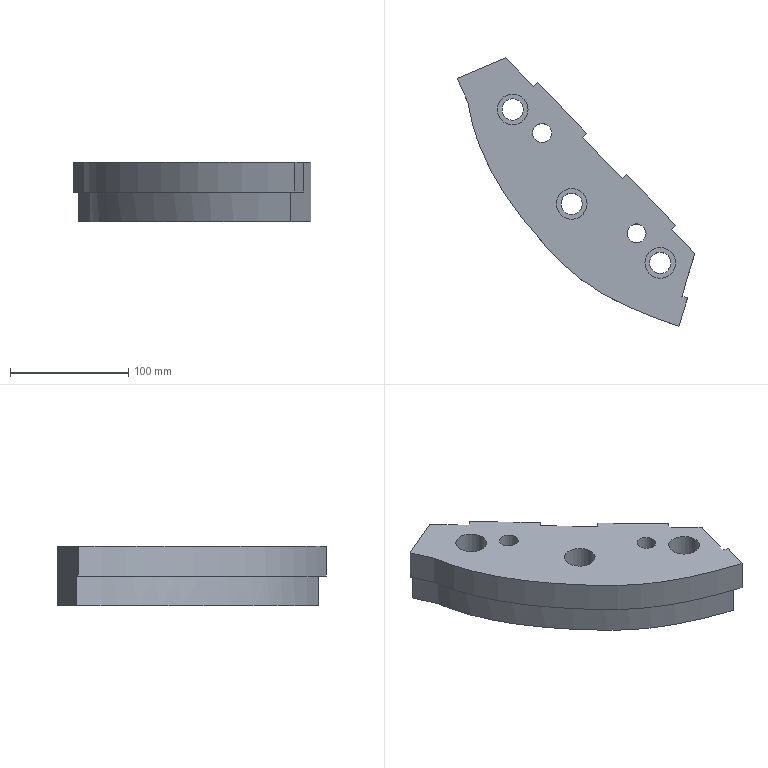Part | NX | features solid 2 | 1 solid | 29 faces | box 201.367 x 227.4 x 50 mm | volume 876647 mm3 | plane 18 | cylinder 8 | spline 3 | commonest cylinder face diameters 18 x3 26 x3 16 x2
STEP:
#1=CARTESIAN_POINT('',(-598.221,-127.253,-50.));
#2=VERTEX_POINT('',#1);
#3=CARTESIAN_POINT('',(-606.221,-127.253,-50.));
#4=DIRECTION('',(0.,0.,1.));
#5=DIRECTION('',(1.,0.,0.));
#6=AXIS2_PLACEMENT_3D('',#3,#4,#5);
#7=CIRCLE('',#6,8.);
#8=EDGE_CURVE('',#2,#2,#7,.F.);
#9=ORIENTED_EDGE('',*,*,#8,.F.);
#10=EDGE_LOOP('',(#9));
#11=FACE_BOUND('',#10,.T.);
#12=CARTESIAN_POINT('',(-678.221,-42.253,-50.));
#13=VERTEX_POINT('',#12);
#14=CARTESIAN_POINT('',(-686.221,-42.253,-50.));
#15=DIRECTION('',(0.,0.,1.));
#16=DIRECTION('',(1.,0.,0.));
#17=AXIS2_PLACEMENT_3D('',#14,#15,#16);
#18=CIRCLE('',#17,8.);
#19=EDGE_CURVE('',#13,#13,#18,.F.);
#20=ORIENTED_EDGE('',*,*,#19,.F.);
#21=EDGE_LOOP('',(#20));
#22=FACE_BOUND('',#21,.T.);
#23=CARTESIAN_POINT('',(-753.635,6.009,-50.));
#24=VERTEX_POINT('',#23);
#25=CARTESIAN_POINT('',(-717.151,21.495,-50.));
#26=VERTEX_POINT('',#25);
#27=CARTESIAN_POINT('',(-1088.176,-135.995,-50.));
#28=DIRECTION('',(0.9205,0.3907,0.));
#29=VECTOR('',#28,1000.);
#30=LINE('',#27,#29);
#31=EDGE_CURVE('',#24,#26,#30,.T.);
#32=ORIENTED_EDGE('',*,*,#31,.T.);
#33=CARTESIAN_POINT('',(-693.858,-2.626,-50.));
#34=VERTEX_POINT('',#33);
#35=CARTESIAN_POINT('',(-475.644,-228.593,-50.));
#36=DIRECTION('',(0.6947,-0.7193,0.));
#37=VECTOR('',#36,1000.);
#38=LINE('',#35,#37);
#39=EDGE_CURVE('',#26,#34,#38,.T.);
#40=ORIENTED_EDGE('',*,*,#39,.T.);
#41=CARTESIAN_POINT('',(-690.261,0.8474,-50.));
#42=VERTEX_POINT('',#41);
#43=CARTESIAN_POINT('',(-683.068,7.794,-50.));
#44=DIRECTION('',(0.7193,0.6947,0.));
#45=VECTOR('',#44,1000.);
#46=LINE('',#43,#45);
#47=EDGE_CURVE('',#34,#42,#46,.T.);
#48=ORIENTED_EDGE('',*,*,#47,.T.);
#49=CARTESIAN_POINT('',(-648.581,-42.313,-50.));
#50=VERTEX_POINT('',#49);
#51=CARTESIAN_POINT('',(-472.047,-225.12,-50.));
#52=DIRECTION('',(0.6947,-0.7193,0.));
#53=VECTOR('',#52,1000.);
#54=LINE('',#51,#53);
#55=EDGE_CURVE('',#42,#50,#54,.T.);
#56=ORIENTED_EDGE('',*,*,#55,.T.);
#57=CARTESIAN_POINT('',(-652.178,-45.786,-50.));
#58=VERTEX_POINT('',#57);
#59=CARTESIAN_POINT('',(-641.388,-35.366,-50.));
#60=DIRECTION('',(0.7193,0.6947,0.));
#61=VECTOR('',#60,1000.);
#62=LINE('',#59,#61);
#63=EDGE_CURVE('',#58,#50,#62,.T.);
#64=ORIENTED_EDGE('',*,*,#63,.F.);
#65=CARTESIAN_POINT('',(-618.219,-80.952,-50.));
#66=VERTEX_POINT('',#65);
#67=CARTESIAN_POINT('',(-475.644,-228.593,-50.));
#68=DIRECTION('',(0.6947,-0.7193,0.));
#69=VECTOR('',#68,1000.);
#70=LINE('',#67,#69);
#71=EDGE_CURVE('',#58,#66,#70,.T.);
#72=ORIENTED_EDGE('',*,*,#71,.T.);
#73=CARTESIAN_POINT('',(-614.622,-77.479,-50.));
#74=VERTEX_POINT('',#73);
#75=CARTESIAN_POINT('',(-607.429,-70.532,-50.));
#76=DIRECTION('',(0.7193,0.6947,0.));
#77=VECTOR('',#76,1000.);
#78=LINE('',#75,#77);
#79=EDGE_CURVE('',#66,#74,#78,.T.);
#80=ORIENTED_EDGE('',*,*,#79,.T.);
#81=CARTESIAN_POINT('',(-572.943,-120.639,-50.));
#82=VERTEX_POINT('',#81);
#83=CARTESIAN_POINT('',(-472.047,-225.12,-50.));
#84=DIRECTION('',(0.6947,-0.7193,0.));
#85=VECTOR('',#84,1000.);
#86=LINE('',#83,#85);
#87=EDGE_CURVE('',#74,#82,#86,.T.);
#88=ORIENTED_EDGE('',*,*,#87,.T.);
#89=CARTESIAN_POINT('',(-576.539,-124.112,-50.));
#90=VERTEX_POINT('',#89);
#91=CARTESIAN_POINT('',(-565.749,-113.693,-50.));
#92=DIRECTION('',(0.7193,0.6947,0.));
#93=VECTOR('',#92,1000.);
#94=LINE('',#91,#93);
#95=EDGE_CURVE('',#90,#82,#94,.T.);
#96=ORIENTED_EDGE('',*,*,#95,.F.);
#97=CARTESIAN_POINT('',(-556.873,-144.478,-50.));
#98=VERTEX_POINT('',#97);
#99=CARTESIAN_POINT('',(-475.644,-228.593,-50.));
#100=DIRECTION('',(0.6947,-0.7193,0.));
#101=VECTOR('',#100,1000.);
#102=LINE('',#99,#101);
#103=EDGE_CURVE('',#90,#98,#102,.T.);
#104=ORIENTED_EDGE('',*,*,#103,.T.);
#105=CARTESIAN_POINT('',(-573.715,-199.565,-50.));
#106=VERTEX_POINT('',#105);
#107=CARTESIAN_POINT('',(-717.976,-671.424,-50.));
#108=DIRECTION('',(0.2924,0.9563,0.));
#109=VECTOR('',#108,1000.);
#110=LINE('',#107,#109);
#111=EDGE_CURVE('',#106,#98,#110,.T.);
#112=ORIENTED_EDGE('',*,*,#111,.F.);
#113=CARTESIAN_POINT('',(-573.715,-199.565,-50.));
#114=CARTESIAN_POINT('',(-576.788,-198.542,-50.));
#115=CARTESIAN_POINT('',(-582.785,-196.48,-50.));
#116=CARTESIAN_POINT('',(-589.908,-193.86,-50.));
#117=CARTESIAN_POINT('',(-595.383,-191.738,-50.));
#118=CARTESIAN_POINT('',(-599.375,-190.136,-50.));
#119=CARTESIAN_POINT('',(-602.617,-188.786,-50.));
#120=CARTESIAN_POINT('',(-604.821,-187.843,-50.));
#121=CARTESIAN_POINT('',(-606.091,-187.292,-50.));
#122=CARTESIAN_POINT('',(-606.968,-186.908,-50.));
#123=CARTESIAN_POINT('',(-608.1,-186.407,-50.));
#124=CARTESIAN_POINT('',(-609.511,-185.776,-50.));
#125=CARTESIAN_POINT('',(-611.998,-184.645,-50.));
#126=CARTESIAN_POINT('',(-615.464,-183.016,-50.));
#127=CARTESIAN_POINT('',(-619.529,-181.019,-50.));
#128=CARTESIAN_POINT('',(-624.805,-178.311,-50.));
#129=CARTESIAN_POINT('',(-629.881,-175.522,-50.));
#130=CARTESIAN_POINT('',(-634.12,-173.031,-50.));
#131=CARTESIAN_POINT('',(-636.521,-171.569,-50.));
#132=CARTESIAN_POINT('',(-638.21,-170.518,-50.));
#133=CARTESIAN_POINT('',(-640.201,-169.248,-50.));
#134=CARTESIAN_POINT('',(-642.698,-167.61,-50.));
#135=CARTESIAN_POINT('',(-645.779,-165.508,-50.));
#136=CARTESIAN_POINT('',(-649.35,-162.935,-50.));
#137=CARTESIAN_POINT('',(-652.753,-160.349,-50.));
#138=CARTESIAN_POINT('',(-656.212,-157.564,-50.));
#139=CARTESIAN_POINT('',(-659.605,-154.671,-50.));
#140=CARTESIAN_POINT('',(-662.395,-152.157,-50.));
#141=CARTESIAN_POINT('',(-664.343,-150.328,-50.));
#142=CARTESIAN_POINT('',(-665.429,-149.289,-50.));
#143=CARTESIAN_POINT('',(-666.302,-148.442,-50.));
#144=CARTESIAN_POINT('',(-666.938,-147.817,-50.));
#145=CARTESIAN_POINT('',(-667.89,-146.875,-50.));
#146=CARTESIAN_POINT('',(-669.556,-145.204,-50.));
#147=CARTESIAN_POINT('',(-672.079,-142.613,-50.));
#148=CARTESIAN_POINT('',(-674.748,-139.795,-50.));
#149=CARTESIAN_POINT('',(-676.713,-137.682,-50.));
#150=CARTESIAN_POINT('',(-677.842,-136.458,-50.));
#151=CARTESIAN_POINT('',(-678.75,-135.468,-50.));
#152=CARTESIAN_POINT('',(-679.481,-134.666,-50.));
#153=CARTESIAN_POINT('',(-680.512,-133.531,-50.));
#154=CARTESIAN_POINT('',(-682.275,-131.573,-50.));
#155=CARTESIAN_POINT('',(-684.778,-128.749,-50.));
#156=CARTESIAN_POINT('',(-687.216,-125.939,-50.));
#157=CARTESIAN_POINT('',(-689.168,-123.651,-50.));
#158=CARTESIAN_POINT('',(-690.541,-122.024,-50.));
#159=CARTESIAN_POINT('',(-692.193,-120.044,-50.));
#160=CARTESIAN_POINT('',(-694.26,-117.531,-50.));
#161=CARTESIAN_POINT('',(-697.843,-113.087,-50.));
#162=CARTESIAN_POINT('',(-702.701,-106.8,-50.));
#163=CARTESIAN_POINT('',(-708.165,-99.29,-50.));
#164=CARTESIAN_POINT('',(-713.251,-91.833,-50.));
#165=CARTESIAN_POINT('',(-717.962,-84.424,-50.));
#166=CARTESIAN_POINT('',(-721.573,-78.291,-50.));
#167=CARTESIAN_POINT('',(-724.275,-73.408,-50.));
#168=CARTESIAN_POINT('',(-726.206,-69.761,-50.));
#169=CARTESIAN_POINT('',(-727.742,-66.722,-50.));
#170=CARTESIAN_POINT('',(-728.767,-64.619,-50.));
#171=CARTESIAN_POINT('',(-729.354,-63.39,-50.));
#172=CARTESIAN_POINT('',(-729.751,-62.551,-50.));
#173=CARTESIAN_POINT('',(-730.287,-61.398,-50.));
#174=CARTESIAN_POINT('',(-730.94,-59.973,-50.));
#175=CARTESIAN_POINT('',(-732.076,-57.432,-50.));
#176=CARTESIAN_POINT('',(-733.601,-53.843,-50.));
#177=CARTESIAN_POINT('',(-735.301,-49.544,-50.));
#178=CARTESIAN_POINT('',(-737.383,-43.847,-50.));
#179=CARTESIAN_POINT('',(-739.193,-38.183,-50.));
#180=CARTESIAN_POINT('',(-740.536,-33.281,-50.));
#181=CARTESIAN_POINT('',(-741.239,-30.466,-50.));
#182=CARTESIAN_POINT('',(-741.719,-28.428,-50.));
#183=CARTESIAN_POINT('',(-742.22,-26.135,-50.));
#184=CARTESIAN_POINT('',(-742.668,-23.895,-50.));
#185=CARTESIAN_POINT('',(-743.085,-21.629,-50.));
#186=CARTESIAN_POINT('',(-743.4,-19.725,-50.));
#187=CARTESIAN_POINT('',(-743.636,-18.217,-50.));
#188=CARTESIAN_POINT('',(-743.802,-17.013,-50.));
#189=CARTESIAN_POINT('',(-743.972,-16.088,-50.));
#190=CARTESIAN_POINT('',(-744.359,-14.775,-50.));
#191=CARTESIAN_POINT('',(-744.695,-13.855,-50.));
#192=CARTESIAN_POINT('',(-745.193,-12.697,-50.));
#193=CARTESIAN_POINT('',(-745.585,-11.868,-50.));
#194=CARTESIAN_POINT('',(-745.882,-11.249,-50.));
#195=CARTESIAN_POINT('',(-746.037,-10.929,-50.));
#196=CARTESIAN_POINT('',(-746.198,-10.602,-50.));
#197=CARTESIAN_POINT('',(-746.192,-10.61,-50.));
#198=CARTESIAN_POINT('',(-746.298,-10.385,-50.));
#199=CARTESIAN_POINT('',(-746.421,-10.121,-50.));
#200=CARTESIAN_POINT('',(-746.539,-9.866,-50.));
#201=CARTESIAN_POINT('',(-746.666,-9.591,-50.));
#202=CARTESIAN_POINT('',(-746.708,-9.5,-50.));
#203=CARTESIAN_POINT('',(-746.794,-9.315,-50.));
#204=CARTESIAN_POINT('',(-746.893,-9.102,-50.));
#205=CARTESIAN_POINT('',(-747.01,-8.851,-50.));
#206=CARTESIAN_POINT('',(-747.146,-8.557,-50.));
#207=CARTESIAN_POINT('',(-747.205,-8.431,-50.));
#208=CARTESIAN_POINT('',(-747.331,-8.16,-50.));
#209=CARTESIAN_POINT('',(-747.51,-7.777,-50.));
#210=CARTESIAN_POINT('',(-747.773,-7.213,-50.));
#211=CARTESIAN_POINT('',(-748.214,-6.269,-50.));
#212=CARTESIAN_POINT('',(-748.706,-5.215,-50.));
#213=CARTESIAN_POINT('',(-749.228,-4.092,-50.));
#214=CARTESIAN_POINT('',(-749.59,-3.309,-50.));
#215=CARTESIAN_POINT('',(-749.861,-2.721,-50.));
#216=CARTESIAN_POINT('',(-749.995,-2.431,-50.));
#217=CARTESIAN_POINT('',(-750.304,-1.756,-50.));
#218=CARTESIAN_POINT('',(-750.644,-1.005,-50.));
#219=CARTESIAN_POINT('',(-751.249,0.341,-50.));
#220=CARTESIAN_POINT('',(-752.352,2.858,-50.));
#221=CARTESIAN_POINT('',(-753.162,4.809,-50.));
#222=CARTESIAN_POINT('',(-753.635,6.009,-50.));
#223=B_SPLINE_CURVE_WITH_KNOTS('',3,(#113,#114,#115,#116,#117,#118,#119,#120,#121,#122,#123,#124,#125,#126,#127,#128,#129,#130,#131,#132,#133,#134,#135,#136,#137,#138,#139,#140,#141,#142,#143,#144,#145,#146,#147,#148,#149,#150,#151,#152,#153,#154,#155,#156,#157,#158,#159,#160,#161,#162,#163,#164,#165,#166,#167,#168,#169,#170,#171,#172,#173,#174,#175,#176,#177,#178,#179,#180,#181,#182,#183,#184,#185,#186,#187,#188,#189,#190,#191,#192,#193,#194,#195,#196,#197,#198,#199,#200,#201,#202,#203,#204,#205,#206,#207,#208,#209,#210,#211,#212,#213,#214,#215,#216,#217,#218,#219,#220,#221,#222),.UNSPECIFIED.,.F.,.F.,(4,1,1,1,1,1,1,1,1,1,1,1,1,1,1,1,1,1,1,1,1,1,1,1,1,1,1,1,1,1,1,1,1,1,1,1,1,1,1,1,1,1,1,1,1,1,1,1,1,1,1,1,1,1,1,1,1,1,1,1,1,1,1,1,1,1,1,1,1,1,1,1,1,1,1,1,1,1,1,1,1,1,1,1,1,1,1,1,1,1,1,1,1,1,1,1,1,1,1,1,1,1,1,1,1,1,1,4),(0.,0.03125,0.0625,0.07812,0.09375,0.1094,0.1172,0.1211,0.125,0.1289,0.1328,0.1406,0.1562,0.1719,0.1875,0.2188,0.2344,0.2422,0.25,0.2578,0.2656,0.2812,0.2969,0.3125,0.3281,0.3438,0.3594,0.3672,0.3711,0.375,0.3789,0.3828,0.3906,0.4062,0.4219,0.4297,0.4336,0.4375,0.4414,0.4453,0.4531,0.4688,0.4844,0.4922,0.5,0.5078,0.5156,0.5312,0.5625,0.5938,0.625,0.6562,0.6875,0.7031,0.7188,0.7344,0.7422,0.7461,0.75,0.7539,0.7578,0.7656,0.7812,0.7969,0.8125,0.8438,0.8594,0.8672,0.875,0.8828,0.8906,0.8984,0.9062,0.9102,0.9141,0.918,0.9219,0.9258,0.9297,0.9336,0.9355,0.9365,0.9375,0.9385,0.9395,0.9404,0.9409,0.9414,0.9419,0.9424,0.9434,0.9443,0.9453,0.9463,0.9473,0.9492,0.9512,0.9531,0.957,0.9609,0.9648,0.9668,0.9688,0.9707,0.9727,0.9766,0.9844,1.),.UNSPECIFIED.);
#224=EDGE_CURVE('',#106,#24,#223,.T.);
#225=ORIENTED_EDGE('',*,*,#224,.T.);
#226=EDGE_LOOP('',(#32,#40,#48,#56,#64,#72,#80,#88,#96,#104,#112,#225));
#227=FACE_BOUND('',#226,.T.);
#228=CARTESIAN_POINT('',(-702.221,-22.253,-50.));
#229=VERTEX_POINT('',#228);
#230=CARTESIAN_POINT('',(-711.221,-22.253,-50.));
#231=DIRECTION('',(0.,0.,1.));
#232=DIRECTION('',(1.,0.,0.));
#233=AXIS2_PLACEMENT_3D('',#230,#231,#232);
#234=CIRCLE('',#233,9.);
#235=EDGE_CURVE('',#229,#229,#234,.F.);
#236=ORIENTED_EDGE('',*,*,#235,.F.);
#237=EDGE_LOOP('',(#236));
#238=FACE_BOUND('',#237,.T.);
#239=CARTESIAN_POINT('',(-652.221,-102.253,-50.));
#240=VERTEX_POINT('',#239);
#241=CARTESIAN_POINT('',(-661.221,-102.253,-50.));
#242=DIRECTION('',(0.,0.,1.));
#243=DIRECTION('',(1.,0.,0.));
#244=AXIS2_PLACEMENT_3D('',#241,#242,#243);
#245=CIRCLE('',#244,9.);
#246=EDGE_CURVE('',#240,#240,#245,.F.);
#247=ORIENTED_EDGE('',*,*,#246,.F.);
#248=EDGE_LOOP('',(#247));
#249=FACE_BOUND('',#248,.T.);
#250=CARTESIAN_POINT('',(-577.221,-152.253,-50.));
#251=VERTEX_POINT('',#250);
#252=CARTESIAN_POINT('',(-586.221,-152.253,-50.));
#253=DIRECTION('',(0.,0.,1.));
#254=DIRECTION('',(1.,0.,0.));
#255=AXIS2_PLACEMENT_3D('',#252,#253,#254);
#256=CIRCLE('',#255,9.);
#257=EDGE_CURVE('',#251,#251,#256,.F.);
#258=ORIENTED_EDGE('',*,*,#257,.F.);
#259=EDGE_LOOP('',(#258));
#260=FACE_BOUND('',#259,.T.);
#261=CARTESIAN_POINT('',(-882.213,-621.212,-50.));
#262=DIRECTION('',(0.,0.,1.));
#263=DIRECTION('',(1.,0.,0.));
#264=AXIS2_PLACEMENT_3D('',#261,#262,#263);
#265=PLANE('',#264);
#266=ADVANCED_FACE('',(#11,#22,#227,#238,#249,#260),#265,.F.);
#267=CARTESIAN_POINT('',(-618.219,-80.952,0.));
#268=VERTEX_POINT('',#267);
#269=CARTESIAN_POINT('',(-618.219,-80.952,-25.));
#270=DIRECTION('',(0.,0.,-1.));
#271=VECTOR('',#270,1000.);
#272=LINE('',#269,#271);
#273=EDGE_CURVE('',#268,#66,#272,.T.);
#274=ORIENTED_EDGE('',*,*,#273,.T.);
#275=ORIENTED_EDGE('',*,*,#71,.F.);
#276=CARTESIAN_POINT('',(-652.178,-45.786,0.));
#277=VERTEX_POINT('',#276);
#278=CARTESIAN_POINT('',(-652.178,-45.786,-25.));
#279=DIRECTION('',(0.,0.,-1.));
#280=VECTOR('',#279,1000.);
#281=LINE('',#278,#280);
#282=EDGE_CURVE('',#277,#58,#281,.T.);
#283=ORIENTED_EDGE('',*,*,#282,.F.);
#284=CARTESIAN_POINT('',(-711.018,15.144,0.));
#285=DIRECTION('',(0.6947,-0.7193,0.));
#286=VECTOR('',#285,1000.);
#287=LINE('',#284,#286);
#288=EDGE_CURVE('',#277,#268,#287,.T.);
#289=ORIENTED_EDGE('',*,*,#288,.T.);
#290=EDGE_LOOP('',(#274,#275,#283,#289));
#291=FACE_BOUND('',#290,.T.);
#292=CARTESIAN_POINT('',(-711.018,15.144,-25.));
#293=DIRECTION('',(-0.7193,-0.6947,0.));
#294=DIRECTION('',(0.6947,-0.7193,0.));
#295=AXIS2_PLACEMENT_3D('',#292,#293,#294);
#296=PLANE('',#295);
#297=ADVANCED_FACE('',(#291),#296,.F.);
#298=CARTESIAN_POINT('',(-693.858,-2.626,0.));
#299=VERTEX_POINT('',#298);
#300=CARTESIAN_POINT('',(-693.858,-2.626,-25.));
#301=DIRECTION('',(0.,0.,-1.));
#302=VECTOR('',#301,1000.);
#303=LINE('',#300,#302);
#304=EDGE_CURVE('',#299,#34,#303,.T.);
#305=ORIENTED_EDGE('',*,*,#304,.T.);
#306=ORIENTED_EDGE('',*,*,#39,.F.);
#307=CARTESIAN_POINT('',(-717.151,21.495,0.));
#308=VERTEX_POINT('',#307);
#309=CARTESIAN_POINT('',(-717.151,21.495,-25.));
#310=DIRECTION('',(0.,0.,1.));
#311=VECTOR('',#310,1000.);
#312=LINE('',#309,#311);
#313=EDGE_CURVE('',#26,#308,#312,.T.);
#314=ORIENTED_EDGE('',*,*,#313,.T.);
#315=CARTESIAN_POINT('',(-711.018,15.144,0.));
#316=DIRECTION('',(0.6947,-0.7193,0.));
#317=VECTOR('',#316,1000.);
#318=LINE('',#315,#317);
#319=EDGE_CURVE('',#308,#299,#318,.T.);
#320=ORIENTED_EDGE('',*,*,#319,.T.);
#321=EDGE_LOOP('',(#305,#306,#314,#320));
#322=FACE_BOUND('',#321,.T.);
#323=CARTESIAN_POINT('',(-711.018,15.144,-25.));
#324=DIRECTION('',(-0.7193,-0.6947,0.));
#325=DIRECTION('',(0.6947,-0.7193,0.));
#326=AXIS2_PLACEMENT_3D('',#323,#324,#325);
#327=PLANE('',#326);
#328=ADVANCED_FACE('',(#322),#327,.F.);
#329=CARTESIAN_POINT('',(-563.114,-181.994,0.));
#330=VERTEX_POINT('',#329);
#331=CARTESIAN_POINT('',(-567.865,-180.433,0.));
#332=VERTEX_POINT('',#331);
#333=CARTESIAN_POINT('',(-563.114,-181.994,0.));
#334=CARTESIAN_POINT('',(-564.701,-181.481,0.));
#335=CARTESIAN_POINT('',(-566.285,-180.961,0.));
#336=CARTESIAN_POINT('',(-567.865,-180.433,0.));
#337=B_SPLINE_CURVE_WITH_KNOTS('',3,(#333,#334,#335,#336),.UNSPECIFIED.,.F.,.F.,(4,4),(0.,0.00497),.UNSPECIFIED.);
#338=EDGE_CURVE('',#330,#332,#337,.T.);
#339=ORIENTED_EDGE('',*,*,#338,.T.);
#340=CARTESIAN_POINT('',(-556.873,-144.478,0.));
#341=VERTEX_POINT('',#340);
#342=CARTESIAN_POINT('',(-573.744,-199.661,0.));
#343=DIRECTION('',(-0.2924,-0.9563,0.));
#344=VECTOR('',#343,1000.);
#345=LINE('',#342,#344);
#346=EDGE_CURVE('',#341,#332,#345,.T.);
#347=ORIENTED_EDGE('',*,*,#346,.F.);
#348=CARTESIAN_POINT('',(-576.539,-124.112,0.));
#349=VERTEX_POINT('',#348);
#350=CARTESIAN_POINT('',(-711.018,15.144,0.));
#351=DIRECTION('',(0.6947,-0.7193,0.));
#352=VECTOR('',#351,1000.);
#353=LINE('',#350,#352);
#354=EDGE_CURVE('',#349,#341,#353,.T.);
#355=ORIENTED_EDGE('',*,*,#354,.F.);
#356=CARTESIAN_POINT('',(-572.943,-120.639,0.));
#357=VERTEX_POINT('',#356);
#358=CARTESIAN_POINT('',(-614.246,-160.525,0.));
#359=DIRECTION('',(0.7193,0.6947,0.));
#360=VECTOR('',#359,1000.);
#361=LINE('',#358,#360);
#362=EDGE_CURVE('',#349,#357,#361,.T.);
#363=ORIENTED_EDGE('',*,*,#362,.T.);
#364=CARTESIAN_POINT('',(-614.622,-77.479,0.));
#365=VERTEX_POINT('',#364);
#366=CARTESIAN_POINT('',(-611.149,-81.075,0.));
#367=DIRECTION('',(0.6947,-0.7193,0.));
#368=VECTOR('',#367,1000.);
#369=LINE('',#366,#368);
#370=EDGE_CURVE('',#365,#357,#369,.T.);
#371=ORIENTED_EDGE('',*,*,#370,.F.);
#372=CARTESIAN_POINT('',(-655.926,-117.365,0.));
#373=DIRECTION('',(0.7193,0.6947,0.));
#374=VECTOR('',#373,1000.);
#375=LINE('',#372,#374);
#376=EDGE_CURVE('',#268,#365,#375,.T.);
#377=ORIENTED_EDGE('',*,*,#376,.F.);
#378=ORIENTED_EDGE('',*,*,#288,.F.);
#379=CARTESIAN_POINT('',(-648.581,-42.313,0.));
#380=VERTEX_POINT('',#379);
#381=CARTESIAN_POINT('',(-689.885,-82.199,0.));
#382=DIRECTION('',(0.7193,0.6947,0.));
#383=VECTOR('',#382,1000.);
#384=LINE('',#381,#383);
#385=EDGE_CURVE('',#277,#380,#384,.T.);
#386=ORIENTED_EDGE('',*,*,#385,.T.);
#387=CARTESIAN_POINT('',(-690.261,0.8474,0.));
#388=VERTEX_POINT('',#387);
#389=CARTESIAN_POINT('',(-714.574,26.024,0.));
#390=DIRECTION('',(0.6947,-0.7193,0.));
#391=VECTOR('',#390,1000.);
#392=LINE('',#389,#391);
#393=EDGE_CURVE('',#388,#380,#392,.T.);
#394=ORIENTED_EDGE('',*,*,#393,.F.);
#395=CARTESIAN_POINT('',(-731.564,-39.039,0.));
#396=DIRECTION('',(0.7193,0.6947,0.));
#397=VECTOR('',#396,1000.);
#398=LINE('',#395,#397);
#399=EDGE_CURVE('',#299,#388,#398,.T.);
#400=ORIENTED_EDGE('',*,*,#399,.F.);
#401=ORIENTED_EDGE('',*,*,#319,.F.);
#402=CARTESIAN_POINT('',(-758.239,4.055,0.));
#403=VERTEX_POINT('',#402);
#404=CARTESIAN_POINT('',(-1958.229,-505.311,0.));
#405=DIRECTION('',(0.9205,0.3907,0.));
#406=VECTOR('',#405,1000.);
#407=LINE('',#404,#406);
#408=EDGE_CURVE('',#403,#308,#407,.T.);
#409=ORIENTED_EDGE('',*,*,#408,.F.);
#410=CARTESIAN_POINT('',(-570.424,-205.904,0.));
#411=VERTEX_POINT('',#410);
#412=CARTESIAN_POINT('',(-758.239,4.055,0.));
#413=CARTESIAN_POINT('',(-757.144,1.281,0.));
#414=CARTESIAN_POINT('',(-755.343,-2.817,0.));
#415=CARTESIAN_POINT('',(-752.812,-8.229,0.));
#416=CARTESIAN_POINT('',(-751.252,-11.62,0.));
#417=CARTESIAN_POINT('',(-749.959,-14.316,0.));
#418=CARTESIAN_POINT('',(-749.016,-16.348,0.));
#419=CARTESIAN_POINT('',(-748.615,-18.594,0.));
#420=CARTESIAN_POINT('',(-748.178,-21.629,0.));
#421=CARTESIAN_POINT('',(-747.492,-25.366,0.));
#422=CARTESIAN_POINT('',(-746.238,-31.284,0.));
#423=CARTESIAN_POINT('',(-744.334,-38.548,0.));
#424=CARTESIAN_POINT('',(-740.668,-49.926,0.));
#425=CARTESIAN_POINT('',(-735.009,-63.721,0.));
#426=CARTESIAN_POINT('',(-726.757,-79.698,0.));
#427=CARTESIAN_POINT('',(-717.23,-95.169,0.));
#428=CARTESIAN_POINT('',(-706.569,-110.192,0.));
#429=CARTESIAN_POINT('',(-694.918,-124.823,0.));
#430=CARTESIAN_POINT('',(-682.359,-139.091,0.));
#431=CARTESIAN_POINT('',(-669.418,-152.804,0.));
#432=CARTESIAN_POINT('',(-655.303,-165.141,0.));
#433=CARTESIAN_POINT('',(-639.796,-175.759,0.));
#434=CARTESIAN_POINT('',(-623.086,-185.082,0.));
#435=CARTESIAN_POINT('',(-600.12,-195.69,0.));
#436=CARTESIAN_POINT('',(-582.381,-202.048,0.));
#437=CARTESIAN_POINT('',(-570.424,-205.904,0.));
#438=B_SPLINE_CURVE_WITH_KNOTS('',3,(#412,#413,#414,#415,#416,#417,#418,#419,#420,#421,#422,#423,#424,#425,#426,#427,#428,#429,#430,#431,#432,#433,#434,#435,#436,#437),.UNSPECIFIED.,.F.,.F.,(4,1,1,1,1,1,1,1,1,1,1,1,1,1,1,1,1,1,1,1,1,1,1,4),(1.545,1.554,1.558,1.563,1.565,1.567,1.57,1.572,1.576,1.581,1.59,1.599,1.617,1.635,1.652,1.67,1.688,1.706,1.724,1.742,1.76,1.778,1.796,1.832),.UNSPECIFIED.);
#439=EDGE_CURVE('',#411,#403,#438,.F.);
#440=ORIENTED_EDGE('',*,*,#439,.F.);
#441=CARTESIAN_POINT('',(-976.675,-1534.691,0.));
#442=DIRECTION('',(0.2924,0.9563,0.));
#443=VECTOR('',#442,1000.);
#444=LINE('',#441,#443);
#445=EDGE_CURVE('',#411,#330,#444,.T.);
#446=ORIENTED_EDGE('',*,*,#445,.T.);
#447=EDGE_LOOP('',(#339,#347,#355,#363,#371,#377,#378,#386,#394,#400,#401,#409,#440,#446));
#448=FACE_BOUND('',#447,.T.);
#449=CARTESIAN_POINT('',(-648.221,-102.253,0.));
#450=VERTEX_POINT('',#449);
#451=CARTESIAN_POINT('',(-661.221,-102.253,0.));
#452=DIRECTION('',(0.,0.,1.));
#453=DIRECTION('',(1.,0.,0.));
#454=AXIS2_PLACEMENT_3D('',#451,#452,#453);
#455=CIRCLE('',#454,13.);
#456=EDGE_CURVE('',#450,#450,#455,.F.);
#457=ORIENTED_EDGE('',*,*,#456,.T.);
#458=EDGE_LOOP('',(#457));
#459=FACE_BOUND('',#458,.T.);
#460=CARTESIAN_POINT('',(-678.221,-42.253,0.));
#461=VERTEX_POINT('',#460);
#462=CARTESIAN_POINT('',(-686.221,-42.253,0.));
#463=DIRECTION('',(0.,0.,1.));
#464=DIRECTION('',(1.,0.,0.));
#465=AXIS2_PLACEMENT_3D('',#462,#463,#464);
#466=CIRCLE('',#465,8.);
#467=EDGE_CURVE('',#461,#461,#466,.F.);
#468=ORIENTED_EDGE('',*,*,#467,.T.);
#469=EDGE_LOOP('',(#468));
#470=FACE_BOUND('',#469,.T.);
#471=CARTESIAN_POINT('',(-598.221,-127.253,0.));
#472=VERTEX_POINT('',#471);
#473=CARTESIAN_POINT('',(-606.221,-127.253,0.));
#474=DIRECTION('',(0.,0.,1.));
#475=DIRECTION('',(1.,0.,0.));
#476=AXIS2_PLACEMENT_3D('',#473,#474,#475);
#477=CIRCLE('',#476,8.);
#478=EDGE_CURVE('',#472,#472,#477,.F.);
#479=ORIENTED_EDGE('',*,*,#478,.T.);
#480=EDGE_LOOP('',(#479));
#481=FACE_BOUND('',#480,.T.);
#482=CARTESIAN_POINT('',(-698.221,-22.253,0.));
#483=VERTEX_POINT('',#482);
#484=CARTESIAN_POINT('',(-711.221,-22.253,0.));
#485=DIRECTION('',(0.,0.,1.));
#486=DIRECTION('',(1.,0.,0.));
#487=AXIS2_PLACEMENT_3D('',#484,#485,#486);
#488=CIRCLE('',#487,13.);
#489=EDGE_CURVE('',#483,#483,#488,.F.);
#490=ORIENTED_EDGE('',*,*,#489,.T.);
#491=EDGE_LOOP('',(#490));
#492=FACE_BOUND('',#491,.T.);
#493=CARTESIAN_POINT('',(-573.221,-152.253,0.));
#494=VERTEX_POINT('',#493);
#495=CARTESIAN_POINT('',(-586.221,-152.253,0.));
#496=DIRECTION('',(0.,0.,1.));
#497=DIRECTION('',(1.,0.,0.));
#498=AXIS2_PLACEMENT_3D('',#495,#496,#497);
#499=CIRCLE('',#498,13.);
#500=EDGE_CURVE('',#494,#494,#499,.F.);
#501=ORIENTED_EDGE('',*,*,#500,.T.);
#502=EDGE_LOOP('',(#501));
#503=FACE_BOUND('',#502,.T.);
#504=CARTESIAN_POINT('',(-688.275,33.753,0.));
#505=DIRECTION('',(0.,0.,-1.));
#506=DIRECTION('',(-1.,0.,0.));
#507=AXIS2_PLACEMENT_3D('',#504,#505,#506);
#508=PLANE('',#507);
#509=ADVANCED_FACE('',(#448,#459,#470,#481,#492,#503),#508,.F.);
#510=CARTESIAN_POINT('',(-556.873,-144.478,-70.));
#511=DIRECTION('',(0.,0.,-1.));
#512=VECTOR('',#511,1000.);
#513=LINE('',#510,#512);
#514=EDGE_CURVE('',#341,#98,#513,.T.);
#515=ORIENTED_EDGE('',*,*,#514,.F.);
#516=ORIENTED_EDGE('',*,*,#346,.T.);
#517=CARTESIAN_POINT('',(-567.865,-180.433,-25.));
#518=VERTEX_POINT('',#517);
#519=CARTESIAN_POINT('',(-567.865,-180.433,-25.));
#520=DIRECTION('',(0.,0.,-1.));
#521=VECTOR('',#520,1000.);
#522=LINE('',#519,#521);
#523=EDGE_CURVE('',#518,#332,#522,.F.);
#524=ORIENTED_EDGE('',*,*,#523,.F.);
#525=CARTESIAN_POINT('',(-573.715,-199.565,-25.));
#526=VERTEX_POINT('',#525);
#527=CARTESIAN_POINT('',(-573.744,-199.661,-25.));
#528=DIRECTION('',(0.2924,0.9563,0.));
#529=VECTOR('',#528,1000.);
#530=LINE('',#527,#529);
#531=EDGE_CURVE('',#526,#518,#530,.T.);
#532=ORIENTED_EDGE('',*,*,#531,.F.);
#533=CARTESIAN_POINT('',(-573.715,-199.565,-42.5));
#534=DIRECTION('',(0.,0.,1.));
#535=VECTOR('',#534,1000.);
#536=LINE('',#533,#535);
#537=EDGE_CURVE('',#526,#106,#536,.F.);
#538=ORIENTED_EDGE('',*,*,#537,.T.);
#539=ORIENTED_EDGE('',*,*,#111,.T.);
#540=EDGE_LOOP('',(#515,#516,#524,#532,#538,#539));
#541=FACE_BOUND('',#540,.T.);
#542=CARTESIAN_POINT('',(-573.744,-199.661,-70.));
#543=DIRECTION('',(0.9563,-0.2924,0.));
#544=DIRECTION('',(0.2924,0.9563,0.));
#545=AXIS2_PLACEMENT_3D('',#542,#543,#544);
#546=PLANE('',#545);
#547=ADVANCED_FACE('',(#541),#546,.T.);
#548=CARTESIAN_POINT('',(-563.114,-181.994,-25.));
#549=VERTEX_POINT('',#548);
#550=CARTESIAN_POINT('',(-563.114,-181.994,-25.));
#551=CARTESIAN_POINT('',(-564.705,-181.48,-25.));
#552=CARTESIAN_POINT('',(-566.288,-180.96,-25.));
#553=CARTESIAN_POINT('',(-567.865,-180.433,-25.));
#554=B_SPLINE_CURVE_WITH_KNOTS('',3,(#550,#551,#552,#553),.UNSPECIFIED.,.F.,.F.,(4,4),(0.001623,0.02295),.UNSPECIFIED.);
#555=EDGE_CURVE('',#549,#518,#554,.T.);
#556=ORIENTED_EDGE('',*,*,#555,.F.);
#557=CARTESIAN_POINT('',(-570.424,-205.904,-25.));
#558=VERTEX_POINT('',#557);
#559=CARTESIAN_POINT('',(-976.675,-1534.691,-25.));
#560=DIRECTION('',(0.2924,0.9563,0.));
#561=VECTOR('',#560,1000.);
#562=LINE('',#559,#561);
#563=EDGE_CURVE('',#558,#549,#562,.T.);
#564=ORIENTED_EDGE('',*,*,#563,.F.);
#565=CARTESIAN_POINT('',(-758.239,4.055,-25.));
#566=VERTEX_POINT('',#565);
#567=CARTESIAN_POINT('',(-758.239,4.055,-25.));
#568=CARTESIAN_POINT('',(-757.142,1.278,-25.));
#569=CARTESIAN_POINT('',(-755.34,-2.825,-25.));
#570=CARTESIAN_POINT('',(-752.804,-8.244,-25.));
#571=CARTESIAN_POINT('',(-751.243,-11.64,-25.));
#572=CARTESIAN_POINT('',(-749.947,-14.338,-25.));
#573=CARTESIAN_POINT('',(-749.007,-16.374,-25.));
#574=CARTESIAN_POINT('',(-748.612,-18.625,-25.));
#575=CARTESIAN_POINT('',(-748.172,-21.66,-25.));
#576=CARTESIAN_POINT('',(-747.485,-25.4,-25.));
#577=CARTESIAN_POINT('',(-746.229,-31.321,-25.));
#578=CARTESIAN_POINT('',(-744.322,-38.591,-25.));
#579=CARTESIAN_POINT('',(-740.648,-49.978,-25.));
#580=CARTESIAN_POINT('',(-734.978,-63.788,-25.));
#581=CARTESIAN_POINT('',(-726.709,-79.784,-25.));
#582=CARTESIAN_POINT('',(-717.158,-95.277,-25.));
#583=CARTESIAN_POINT('',(-706.476,-110.316,-25.));
#584=CARTESIAN_POINT('',(-694.776,-124.992,-25.));
#585=CARTESIAN_POINT('',(-682.253,-139.205,-25.));
#586=CARTESIAN_POINT('',(-669.354,-152.867,-25.));
#587=CARTESIAN_POINT('',(-655.25,-165.181,-25.));
#588=CARTESIAN_POINT('',(-639.704,-175.817,-25.));
#589=CARTESIAN_POINT('',(-622.973,-185.138,-25.));
#590=CARTESIAN_POINT('',(-600.103,-195.693,-25.));
#591=CARTESIAN_POINT('',(-582.374,-202.05,-25.));
#592=CARTESIAN_POINT('',(-570.424,-205.904,-25.));
#593=B_SPLINE_CURVE_WITH_KNOTS('',3,(#567,#568,#569,#570,#571,#572,#573,#574,#575,#576,#577,#578,#579,#580,#581,#582,#583,#584,#585,#586,#587,#588,#589,#590,#591,#592),.UNSPECIFIED.,.F.,.F.,(4,1,1,1,1,1,1,1,1,1,1,1,1,1,1,1,1,1,1,1,1,1,1,4),(1.469,1.478,1.483,1.487,1.49,1.492,1.494,1.496,1.501,1.505,1.514,1.523,1.541,1.559,1.577,1.595,1.613,1.631,1.649,1.667,1.685,1.703,1.721,1.756),.UNSPECIFIED.);
#594=EDGE_CURVE('',#558,#566,#593,.F.);
#595=ORIENTED_EDGE('',*,*,#594,.T.);
#596=CARTESIAN_POINT('',(-753.635,6.009,-25.));
#597=VERTEX_POINT('',#596);
#598=CARTESIAN_POINT('',(-1958.229,-505.311,-25.));
#599=DIRECTION('',(0.9205,0.3907,0.));
#600=VECTOR('',#599,1000.);
#601=LINE('',#598,#600);
#602=EDGE_CURVE('',#566,#597,#601,.T.);
#603=ORIENTED_EDGE('',*,*,#602,.T.);
#604=CARTESIAN_POINT('',(-573.715,-199.565,-25.));
#605=CARTESIAN_POINT('',(-585.053,-195.791,-25.));
#606=CARTESIAN_POINT('',(-601.795,-189.572,-25.));
#607=CARTESIAN_POINT('',(-623.22,-179.362,-25.));
#608=CARTESIAN_POINT('',(-638.713,-170.517,-25.));
#609=CARTESIAN_POINT('',(-653.546,-160.162,-25.));
#610=CARTESIAN_POINT('',(-667.029,-148.094,-25.));
#611=CARTESIAN_POINT('',(-679.251,-135.061,-25.));
#612=CARTESIAN_POINT('',(-691.016,-121.671,-25.));
#613=CARTESIAN_POINT('',(-702.118,-107.769,-25.));
#614=CARTESIAN_POINT('',(-712.47,-93.281,-25.));
#615=CARTESIAN_POINT('',(-721.91,-78.111,-25.));
#616=CARTESIAN_POINT('',(-730.292,-62.032,-25.));
#617=CARTESIAN_POINT('',(-735.995,-48.165,-25.));
#618=CARTESIAN_POINT('',(-739.655,-36.74,-25.));
#619=CARTESIAN_POINT('',(-741.539,-29.452,-25.));
#620=CARTESIAN_POINT('',(-742.753,-23.514,-25.));
#621=CARTESIAN_POINT('',(-743.43,-19.773,-25.));
#622=CARTESIAN_POINT('',(-743.809,-16.72,-25.));
#623=CARTESIAN_POINT('',(-744.591,-13.815,-25.));
#624=CARTESIAN_POINT('',(-746.303,-10.453,-25.));
#625=CARTESIAN_POINT('',(-748.166,-6.348,-25.));
#626=CARTESIAN_POINT('',(-750.725,-0.9033,-25.));
#627=CARTESIAN_POINT('',(-752.534,3.221,-25.));
#628=CARTESIAN_POINT('',(-753.635,6.009,-25.));
#629=B_SPLINE_CURVE_WITH_KNOTS('',3,(#604,#605,#606,#607,#608,#609,#610,#611,#612,#613,#614,#615,#616,#617,#618,#619,#620,#621,#622,#623,#624,#625,#626,#627,#628),.UNSPECIFIED.,.F.,.F.,(4,1,1,1,1,1,1,1,1,1,1,1,1,1,1,1,1,1,1,1,1,1,4),(0.6959,0.7318,0.7497,0.7676,0.7856,0.8035,0.8214,0.8393,0.8573,0.8752,0.8931,0.9111,0.929,0.938,0.9469,0.9514,0.9559,0.9581,0.9604,0.9649,0.9693,0.9738,0.9828),.UNSPECIFIED.);
#630=EDGE_CURVE('',#526,#597,#629,.T.);
#631=ORIENTED_EDGE('',*,*,#630,.F.);
#632=ORIENTED_EDGE('',*,*,#531,.T.);
#633=EDGE_LOOP('',(#556,#564,#595,#603,#631,#632));
#634=FACE_BOUND('',#633,.T.);
#635=CARTESIAN_POINT('',(-570.424,-205.904,-25.));
#636=DIRECTION('',(0.,0.,-1.));
#637=DIRECTION('',(-1.,0.,0.));
#638=AXIS2_PLACEMENT_3D('',#635,#636,#637);
#639=PLANE('',#638);
#640=ADVANCED_FACE('',(#634),#639,.T.);
#641=ORIENTED_EDGE('',*,*,#537,.F.);
#642=ORIENTED_EDGE('',*,*,#630,.T.);
#643=CARTESIAN_POINT('',(-753.635,6.009,-42.5));
#644=DIRECTION('',(0.,0.,1.));
#645=VECTOR('',#644,1000.);
#646=LINE('',#643,#645);
#647=EDGE_CURVE('',#597,#24,#646,.F.);
#648=ORIENTED_EDGE('',*,*,#647,.T.);
#649=ORIENTED_EDGE('',*,*,#224,.F.);
#650=EDGE_LOOP('',(#641,#642,#648,#649));
#651=FACE_BOUND('',#650,.T.);
#652=CARTESIAN_POINT('',(-573.715,-199.565,-50.));
#653=CARTESIAN_POINT('',(-573.715,-199.565,-25.));
#654=CARTESIAN_POINT('',(-585.12,-195.769,-50.));
#655=CARTESIAN_POINT('',(-585.12,-195.769,-25.));
#656=CARTESIAN_POINT('',(-601.987,-189.498,-50.));
#657=CARTESIAN_POINT('',(-601.987,-189.498,-25.));
#658=CARTESIAN_POINT('',(-623.5,-179.217,-50.));
#659=CARTESIAN_POINT('',(-623.5,-179.217,-25.));
#660=CARTESIAN_POINT('',(-638.947,-170.364,-50.));
#661=CARTESIAN_POINT('',(-638.947,-170.364,-25.));
#662=CARTESIAN_POINT('',(-653.471,-160.193,-50.));
#663=CARTESIAN_POINT('',(-653.471,-160.193,-25.));
#664=CARTESIAN_POINT('',(-666.618,-148.499,-50.));
#665=CARTESIAN_POINT('',(-666.618,-148.499,-25.));
#666=CARTESIAN_POINT('',(-678.964,-135.383,-50.));
#667=CARTESIAN_POINT('',(-678.964,-135.383,-25.));
#668=CARTESIAN_POINT('',(-690.853,-121.868,-50.));
#669=CARTESIAN_POINT('',(-690.853,-121.868,-25.));
#670=CARTESIAN_POINT('',(-702.068,-107.84,-50.));
#671=CARTESIAN_POINT('',(-702.068,-107.84,-25.));
#672=CARTESIAN_POINT('',(-712.486,-93.26,-50.));
#673=CARTESIAN_POINT('',(-712.486,-93.26,-25.));
#674=CARTESIAN_POINT('',(-721.918,-78.089,-50.));
#675=CARTESIAN_POINT('',(-721.918,-78.089,-25.));
#676=CARTESIAN_POINT('',(-728.787,-64.923,-50.));
#677=CARTESIAN_POINT('',(-728.787,-64.923,-25.));
#678=CARTESIAN_POINT('',(-733.555,-54.092,-50.));
#679=CARTESIAN_POINT('',(-733.555,-54.092,-25.));
#680=CARTESIAN_POINT('',(-736.724,-45.828,-50.));
#681=CARTESIAN_POINT('',(-736.724,-45.828,-25.));
#682=CARTESIAN_POINT('',(-738.997,-38.828,-50.));
#683=CARTESIAN_POINT('',(-738.997,-38.828,-25.));
#684=CARTESIAN_POINT('',(-740.574,-33.167,-50.));
#685=CARTESIAN_POINT('',(-740.574,-33.167,-25.));
#686=CARTESIAN_POINT('',(-741.629,-28.895,-50.));
#687=CARTESIAN_POINT('',(-741.629,-28.895,-25.));
#688=CARTESIAN_POINT('',(-742.396,-25.315,-50.));
#689=CARTESIAN_POINT('',(-742.396,-25.315,-25.));
#690=CARTESIAN_POINT('',(-742.94,-22.439,-50.));
#691=CARTESIAN_POINT('',(-742.94,-22.439,-25.));
#692=CARTESIAN_POINT('',(-743.251,-20.64,-50.));
#693=CARTESIAN_POINT('',(-743.251,-20.64,-25.));
#694=CARTESIAN_POINT('',(-743.485,-19.181,-50.));
#695=CARTESIAN_POINT('',(-743.485,-19.181,-25.));
#696=CARTESIAN_POINT('',(-743.621,-18.301,-50.));
#697=CARTESIAN_POINT('',(-743.621,-18.301,-25.));
#698=CARTESIAN_POINT('',(-743.718,-17.592,-50.));
#699=CARTESIAN_POINT('',(-743.718,-17.592,-25.));
#700=CARTESIAN_POINT('',(-743.835,-16.823,-50.));
#701=CARTESIAN_POINT('',(-743.835,-16.823,-25.));
#702=CARTESIAN_POINT('',(-744.024,-15.948,-50.));
#703=CARTESIAN_POINT('',(-744.024,-15.948,-25.));
#704=CARTESIAN_POINT('',(-744.32,-14.882,-50.));
#705=CARTESIAN_POINT('',(-744.32,-14.882,-25.));
#706=CARTESIAN_POINT('',(-744.776,-13.621,-50.));
#707=CARTESIAN_POINT('',(-744.776,-13.621,-25.));
#708=CARTESIAN_POINT('',(-745.571,-11.889,-50.));
#709=CARTESIAN_POINT('',(-745.571,-11.889,-25.));
#710=CARTESIAN_POINT('',(-746.307,-10.386,-50.));
#711=CARTESIAN_POINT('',(-746.307,-10.386,-25.));
#712=CARTESIAN_POINT('',(-747.284,-8.253,-50.));
#713=CARTESIAN_POINT('',(-747.284,-8.253,-25.));
#714=CARTESIAN_POINT('',(-748.568,-5.517,-50.));
#715=CARTESIAN_POINT('',(-748.568,-5.517,-25.));
#716=CARTESIAN_POINT('',(-750.158,-2.098,-50.));
#717=CARTESIAN_POINT('',(-750.158,-2.098,-25.));
#718=CARTESIAN_POINT('',(-751.671,1.272,-50.));
#719=CARTESIAN_POINT('',(-751.671,1.272,-25.));
#720=CARTESIAN_POINT('',(-752.825,3.99,-50.));
#721=CARTESIAN_POINT('',(-752.825,3.99,-25.));
#722=CARTESIAN_POINT('',(-753.357,5.303,-50.));
#723=CARTESIAN_POINT('',(-753.357,5.303,-25.));
#724=CARTESIAN_POINT('',(-753.635,6.009,-50.));
#725=CARTESIAN_POINT('',(-753.635,6.009,-25.));
#726=B_SPLINE_SURFACE_WITH_KNOTS('',3,1,((#652,#653),(#654,#655),(#656,#657),(#658,#659),(#660,#661),(#662,#663),(#664,#665),(#666,#667),(#668,#669),(#670,#671),(#672,#673),(#674,#675),(#676,#677),(#678,#679),(#680,#681),(#682,#683),(#684,#685),(#686,#687),(#688,#689),(#690,#691),(#692,#693),(#694,#695),(#696,#697),(#698,#699),(#700,#701),(#702,#703),(#704,#705),(#706,#707),(#708,#709),(#710,#711),(#712,#713),(#714,#715),(#716,#717),(#718,#719),(#720,#721),(#722,#723),(#724,#725)),.SURF_OF_LINEAR_EXTRUSION.,.F.,.F.,.F.,(4,1,1,1,1,1,1,1,1,1,1,1,1,1,1,1,1,1,1,1,1,1,1,1,1,1,1,1,1,1,1,1,1,1,4),(2,2),(0.01729,0.1402,0.2016,0.2631,0.3245,0.386,0.4474,0.5089,0.5703,0.6318,0.6932,0.7546,0.7854,0.8161,0.8468,0.8622,0.8775,0.8929,0.9006,0.9083,0.9121,0.9159,0.9179,0.9198,0.9217,0.9236,0.9275,0.9313,0.939,0.9467,0.9543,0.9697,0.9851,0.9927,1.),(0.,1.),.UNSPECIFIED.);
#727=ADVANCED_FACE('',(#651),#726,.F.);
#728=CARTESIAN_POINT('',(-563.114,-181.994,-12.5));
#729=DIRECTION('',(0.,0.,-1.));
#730=VECTOR('',#729,1000.);
#731=LINE('',#728,#730);
#732=EDGE_CURVE('',#330,#549,#731,.T.);
#733=ORIENTED_EDGE('',*,*,#732,.F.);
#734=ORIENTED_EDGE('',*,*,#445,.F.);
#735=CARTESIAN_POINT('',(-570.424,-205.904,-70.));
#736=DIRECTION('',(0.,0.,1.));
#737=VECTOR('',#736,1000.);
#738=LINE('',#735,#737);
#739=EDGE_CURVE('',#558,#411,#738,.T.);
#740=ORIENTED_EDGE('',*,*,#739,.F.);
#741=ORIENTED_EDGE('',*,*,#563,.T.);
#742=EDGE_LOOP('',(#733,#734,#740,#741));
#743=FACE_BOUND('',#742,.T.);
#744=CARTESIAN_POINT('',(-976.675,-1534.691,-70.));
#745=DIRECTION('',(0.9563,-0.2924,0.));
#746=DIRECTION('',(0.2924,0.9563,0.));
#747=AXIS2_PLACEMENT_3D('',#744,#745,#746);
#748=PLANE('',#747);
#749=ADVANCED_FACE('',(#743),#748,.T.);
#750=ORIENTED_EDGE('',*,*,#408,.T.);
#751=ORIENTED_EDGE('',*,*,#313,.F.);
#752=ORIENTED_EDGE('',*,*,#31,.F.);
#753=ORIENTED_EDGE('',*,*,#647,.F.);
#754=ORIENTED_EDGE('',*,*,#602,.F.);
#755=CARTESIAN_POINT('',(-758.239,4.055,-2.5));
#756=DIRECTION('',(0.,0.,1.));
#757=VECTOR('',#756,1000.);
#758=LINE('',#755,#757);
#759=EDGE_CURVE('',#566,#403,#758,.T.);
#760=ORIENTED_EDGE('',*,*,#759,.T.);
#761=EDGE_LOOP('',(#750,#751,#752,#753,#754,#760));
#762=FACE_BOUND('',#761,.T.);
#763=CARTESIAN_POINT('',(-1958.229,-505.311,-70.));
#764=DIRECTION('',(0.3907,-0.9205,0.));
#765=DIRECTION('',(0.9205,0.3907,0.));
#766=AXIS2_PLACEMENT_3D('',#763,#764,#765);
#767=PLANE('',#766);
#768=ADVANCED_FACE('',(#762),#767,.F.);
#769=ORIENTED_EDGE('',*,*,#594,.F.);
#770=ORIENTED_EDGE('',*,*,#739,.T.);
#771=ORIENTED_EDGE('',*,*,#439,.T.);
#772=ORIENTED_EDGE('',*,*,#759,.F.);
#773=EDGE_LOOP('',(#769,#770,#771,#772));
#774=FACE_BOUND('',#773,.T.);
#775=CARTESIAN_POINT('',(-570.424,-205.904,-25.));
#776=CARTESIAN_POINT('',(-570.424,-205.904,0.));
#777=CARTESIAN_POINT('',(-582.173,-202.115,-25.));
#778=CARTESIAN_POINT('',(-582.173,-202.115,0.));
#779=CARTESIAN_POINT('',(-599.624,-195.869,-25.));
#780=CARTESIAN_POINT('',(-599.624,-195.869,0.));
#781=CARTESIAN_POINT('',(-622.087,-185.568,-25.));
#782=CARTESIAN_POINT('',(-622.087,-185.568,0.));
#783=CARTESIAN_POINT('',(-638.32,-176.644,-25.));
#784=CARTESIAN_POINT('',(-638.32,-176.644,0.));
#785=CARTESIAN_POINT('',(-653.728,-166.321,-25.));
#786=CARTESIAN_POINT('',(-653.728,-166.321,0.));
#787=CARTESIAN_POINT('',(-667.865,-154.321,-25.));
#788=CARTESIAN_POINT('',(-667.865,-154.321,0.));
#789=CARTESIAN_POINT('',(-680.671,-140.922,-25.));
#790=CARTESIAN_POINT('',(-680.671,-140.922,0.));
#791=CARTESIAN_POINT('',(-692.988,-127.095,-25.));
#792=CARTESIAN_POINT('',(-692.988,-127.095,0.));
#793=CARTESIAN_POINT('',(-704.653,-112.705,-25.));
#794=CARTESIAN_POINT('',(-704.653,-112.705,0.));
#795=CARTESIAN_POINT('',(-715.529,-97.708,-25.));
#796=CARTESIAN_POINT('',(-715.529,-97.708,0.));
#797=CARTESIAN_POINT('',(-725.422,-82.043,-25.));
#798=CARTESIAN_POINT('',(-725.422,-82.043,0.));
#799=CARTESIAN_POINT('',(-734.11,-65.669,-25.));
#800=CARTESIAN_POINT('',(-734.11,-65.669,0.));
#801=CARTESIAN_POINT('',(-740.112,-51.431,-25.));
#802=CARTESIAN_POINT('',(-740.112,-51.431,0.));
#803=CARTESIAN_POINT('',(-743.995,-39.713,-25.));
#804=CARTESIAN_POINT('',(-743.995,-39.713,0.));
#805=CARTESIAN_POINT('',(-745.999,-32.258,-25.));
#806=CARTESIAN_POINT('',(-745.999,-32.258,0.));
#807=CARTESIAN_POINT('',(-747.327,-26.23,-25.));
#808=CARTESIAN_POINT('',(-747.327,-26.23,0.));
#809=CARTESIAN_POINT('',(-748.021,-22.433,-25.));
#810=CARTESIAN_POINT('',(-748.021,-22.433,0.));
#811=CARTESIAN_POINT('',(-748.529,-19.392,-25.));
#812=CARTESIAN_POINT('',(-748.529,-19.392,0.));
#813=CARTESIAN_POINT('',(-748.898,-16.31,-25.));
#814=CARTESIAN_POINT('',(-748.898,-16.31,0.));
#815=CARTESIAN_POINT('',(-750.718,-12.848,-25.));
#816=CARTESIAN_POINT('',(-750.718,-12.848,0.));
#817=CARTESIAN_POINT('',(-752.61,-8.64,-25.));
#818=CARTESIAN_POINT('',(-752.61,-8.64,0.));
#819=CARTESIAN_POINT('',(-755.243,-3.051,-25.));
#820=CARTESIAN_POINT('',(-755.243,-3.051,0.));
#821=CARTESIAN_POINT('',(-757.105,1.184,-25.));
#822=CARTESIAN_POINT('',(-757.105,1.184,0.));
#823=CARTESIAN_POINT('',(-758.239,4.055,-25.));
#824=CARTESIAN_POINT('',(-758.239,4.055,0.));
#825=B_SPLINE_SURFACE_WITH_KNOTS('',3,1,((#775,#776),(#777,#778),(#779,#780),(#781,#782),(#783,#784),(#785,#786),(#787,#788),(#789,#790),(#791,#792),(#793,#794),(#795,#796),(#797,#798),(#799,#800),(#801,#802),(#803,#804),(#805,#806),(#807,#808),(#809,#810),(#811,#812),(#813,#814),(#815,#816),(#817,#818),(#819,#820),(#821,#822),(#823,#824)),.SURF_OF_LINEAR_EXTRUSION.,.F.,.F.,.F.,(4,1,1,1,1,1,1,1,1,1,1,1,1,1,1,1,1,1,1,1,1,1,4),(2,2),(0.7427,0.7743,0.7901,0.806,0.8218,0.8376,0.8534,0.8692,0.885,0.9008,0.9166,0.9324,0.9482,0.9561,0.964,0.968,0.9719,0.9739,0.9759,0.9798,0.9838,0.9877,0.9956),(0.,1.),.UNSPECIFIED.);
#826=ADVANCED_FACE('',(#774),#825,.F.);
#827=ORIENTED_EDGE('',*,*,#523,.T.);
#828=ORIENTED_EDGE('',*,*,#338,.F.);
#829=ORIENTED_EDGE('',*,*,#732,.T.);
#830=ORIENTED_EDGE('',*,*,#555,.T.);
#831=EDGE_LOOP('',(#827,#828,#829,#830));
#832=FACE_BOUND('',#831,.T.);
#833=CARTESIAN_POINT('',(-563.114,-181.994,0.));
#834=CARTESIAN_POINT('',(-563.114,-181.994,-25.));
#835=CARTESIAN_POINT('',(-564.705,-181.48,0.));
#836=CARTESIAN_POINT('',(-564.705,-181.48,-25.));
#837=CARTESIAN_POINT('',(-566.288,-180.96,0.));
#838=CARTESIAN_POINT('',(-566.288,-180.96,-25.));
#839=CARTESIAN_POINT('',(-567.865,-180.433,0.));
#840=CARTESIAN_POINT('',(-567.865,-180.433,-25.));
#841=B_SPLINE_SURFACE_WITH_KNOTS('',3,1,((#833,#834),(#835,#836),(#837,#838),(#839,#840)),.SURF_OF_LINEAR_EXTRUSION.,.F.,.F.,.F.,(4,4),(2,2),(0.001623,0.02295),(0.,1.),.PIECEWISE_BEZIER_KNOTS.);
#842=ADVANCED_FACE('',(#832),#841,.F.);
#843=ORIENTED_EDGE('',*,*,#103,.F.);
#844=CARTESIAN_POINT('',(-576.539,-124.112,-25.));
#845=DIRECTION('',(0.,0.,-1.));
#846=VECTOR('',#845,1000.);
#847=LINE('',#844,#846);
#848=EDGE_CURVE('',#349,#90,#847,.T.);
#849=ORIENTED_EDGE('',*,*,#848,.F.);
#850=ORIENTED_EDGE('',*,*,#354,.T.);
#851=ORIENTED_EDGE('',*,*,#514,.T.);
#852=EDGE_LOOP('',(#843,#849,#850,#851));
#853=FACE_BOUND('',#852,.T.);
#854=CARTESIAN_POINT('',(-711.018,15.144,-25.));
#855=DIRECTION('',(-0.7193,-0.6947,0.));
#856=DIRECTION('',(0.6947,-0.7193,0.));
#857=AXIS2_PLACEMENT_3D('',#854,#855,#856);
#858=PLANE('',#857);
#859=ADVANCED_FACE('',(#853),#858,.F.);
#860=CARTESIAN_POINT('',(-648.581,-42.313,-25.));
#861=DIRECTION('',(0.,0.,-1.));
#862=VECTOR('',#861,1000.);
#863=LINE('',#860,#862);
#864=EDGE_CURVE('',#380,#50,#863,.T.);
#865=ORIENTED_EDGE('',*,*,#864,.F.);
#866=ORIENTED_EDGE('',*,*,#385,.F.);
#867=ORIENTED_EDGE('',*,*,#282,.T.);
#868=ORIENTED_EDGE('',*,*,#63,.T.);
#869=EDGE_LOOP('',(#865,#866,#867,#868));
#870=FACE_BOUND('',#869,.T.);
#871=CARTESIAN_POINT('',(-641.388,-35.366,-25.));
#872=DIRECTION('',(0.6947,-0.7193,0.));
#873=DIRECTION('',(0.7193,0.6947,0.));
#874=AXIS2_PLACEMENT_3D('',#871,#872,#873);
#875=PLANE('',#874);
#876=ADVANCED_FACE('',(#870),#875,.T.);
#877=CARTESIAN_POINT('',(-690.261,0.8474,-25.));
#878=DIRECTION('',(0.,0.,-1.));
#879=VECTOR('',#878,1000.);
#880=LINE('',#877,#879);
#881=EDGE_CURVE('',#388,#42,#880,.T.);
#882=ORIENTED_EDGE('',*,*,#881,.T.);
#883=ORIENTED_EDGE('',*,*,#47,.F.);
#884=ORIENTED_EDGE('',*,*,#304,.F.);
#885=ORIENTED_EDGE('',*,*,#399,.T.);
#886=EDGE_LOOP('',(#882,#883,#884,#885));
#887=FACE_BOUND('',#886,.T.);
#888=CARTESIAN_POINT('',(-683.068,7.794,-25.));
#889=DIRECTION('',(0.6947,-0.7193,0.));
#890=DIRECTION('',(0.7193,0.6947,0.));
#891=AXIS2_PLACEMENT_3D('',#888,#889,#890);
#892=PLANE('',#891);
#893=ADVANCED_FACE('',(#887),#892,.F.);
#894=ORIENTED_EDGE('',*,*,#864,.T.);
#895=ORIENTED_EDGE('',*,*,#55,.F.);
#896=ORIENTED_EDGE('',*,*,#881,.F.);
#897=ORIENTED_EDGE('',*,*,#393,.T.);
#898=EDGE_LOOP('',(#894,#895,#896,#897));
#899=FACE_BOUND('',#898,.T.);
#900=CARTESIAN_POINT('',(-714.574,26.024,-25.));
#901=DIRECTION('',(-0.7193,-0.6947,0.));
#902=DIRECTION('',(0.,0.,-1.));
#903=AXIS2_PLACEMENT_3D('',#900,#901,#902);
#904=PLANE('',#903);
#905=ADVANCED_FACE('',(#899),#904,.F.);
#906=CARTESIAN_POINT('',(-572.943,-120.639,-25.));
#907=DIRECTION('',(0.,0.,-1.));
#908=VECTOR('',#907,1000.);
#909=LINE('',#906,#908);
#910=EDGE_CURVE('',#357,#82,#909,.T.);
#911=ORIENTED_EDGE('',*,*,#910,.F.);
#912=ORIENTED_EDGE('',*,*,#362,.F.);
#913=ORIENTED_EDGE('',*,*,#848,.T.);
#914=ORIENTED_EDGE('',*,*,#95,.T.);
#915=EDGE_LOOP('',(#911,#912,#913,#914));
#916=FACE_BOUND('',#915,.T.);
#917=CARTESIAN_POINT('',(-565.749,-113.693,-25.));
#918=DIRECTION('',(0.6947,-0.7193,0.));
#919=DIRECTION('',(0.7193,0.6947,0.));
#920=AXIS2_PLACEMENT_3D('',#917,#918,#919);
#921=PLANE('',#920);
#922=ADVANCED_FACE('',(#916),#921,.T.);
#923=CARTESIAN_POINT('',(-614.622,-77.479,-25.));
#924=DIRECTION('',(0.,0.,-1.));
#925=VECTOR('',#924,1000.);
#926=LINE('',#923,#925);
#927=EDGE_CURVE('',#365,#74,#926,.T.);
#928=ORIENTED_EDGE('',*,*,#927,.T.);
#929=ORIENTED_EDGE('',*,*,#79,.F.);
#930=ORIENTED_EDGE('',*,*,#273,.F.);
#931=ORIENTED_EDGE('',*,*,#376,.T.);
#932=EDGE_LOOP('',(#928,#929,#930,#931));
#933=FACE_BOUND('',#932,.T.);
#934=CARTESIAN_POINT('',(-607.429,-70.532,-25.));
#935=DIRECTION('',(0.6947,-0.7193,0.));
#936=DIRECTION('',(0.7193,0.6947,0.));
#937=AXIS2_PLACEMENT_3D('',#934,#935,#936);
#938=PLANE('',#937);
#939=ADVANCED_FACE('',(#933),#938,.F.);
#940=ORIENTED_EDGE('',*,*,#910,.T.);
#941=ORIENTED_EDGE('',*,*,#87,.F.);
#942=ORIENTED_EDGE('',*,*,#927,.F.);
#943=ORIENTED_EDGE('',*,*,#370,.T.);
#944=EDGE_LOOP('',(#940,#941,#942,#943));
#945=FACE_BOUND('',#944,.T.);
#946=CARTESIAN_POINT('',(-611.149,-81.075,-25.));
#947=DIRECTION('',(-0.7193,-0.6947,0.));
#948=DIRECTION('',(0.,0.,-1.));
#949=AXIS2_PLACEMENT_3D('',#946,#947,#948);
#950=PLANE('',#949);
#951=ADVANCED_FACE('',(#945),#950,.F.);
#952=CARTESIAN_POINT('',(-720.221,-22.253,-30.));
#953=VERTEX_POINT('',#952);
#954=CARTESIAN_POINT('',(-711.221,-22.253,-30.));
#955=DIRECTION('',(0.,0.,-1.));
#956=DIRECTION('',(-1.,0.,0.));
#957=AXIS2_PLACEMENT_3D('',#954,#955,#956);
#958=CIRCLE('',#957,9.);
#959=EDGE_CURVE('',#953,#953,#958,.T.);
#960=ORIENTED_EDGE('',*,*,#959,.F.);
#961=EDGE_LOOP('',(#960));
#962=FACE_BOUND('',#961,.T.);
#963=ORIENTED_EDGE('',*,*,#235,.T.);
#964=EDGE_LOOP('',(#963));
#965=FACE_BOUND('',#964,.T.);
#966=CARTESIAN_POINT('',(-711.221,-22.253,-125.));
#967=DIRECTION('',(0.,0.,1.));
#968=DIRECTION('',(1.,0.,0.));
#969=AXIS2_PLACEMENT_3D('',#966,#967,#968);
#970=CYLINDRICAL_SURFACE('',#969,9.);
#971=ADVANCED_FACE('',(#962,#965),#970,.F.);
#972=ORIENTED_EDGE('',*,*,#467,.F.);
#973=EDGE_LOOP('',(#972));
#974=FACE_BOUND('',#973,.T.);
#975=ORIENTED_EDGE('',*,*,#19,.T.);
#976=EDGE_LOOP('',(#975));
#977=FACE_BOUND('',#976,.T.);
#978=CARTESIAN_POINT('',(-686.221,-42.253,-125.));
#979=DIRECTION('',(0.,0.,1.));
#980=DIRECTION('',(1.,0.,0.));
#981=AXIS2_PLACEMENT_3D('',#978,#979,#980);
#982=CYLINDRICAL_SURFACE('',#981,8.);
#983=ADVANCED_FACE('',(#974,#977),#982,.F.);
#984=CARTESIAN_POINT('',(-670.221,-102.253,-30.));
#985=VERTEX_POINT('',#984);
#986=CARTESIAN_POINT('',(-661.221,-102.253,-30.));
#987=DIRECTION('',(0.,0.,-1.));
#988=DIRECTION('',(-1.,0.,0.));
#989=AXIS2_PLACEMENT_3D('',#986,#987,#988);
#990=CIRCLE('',#989,9.);
#991=EDGE_CURVE('',#985,#985,#990,.T.);
#992=ORIENTED_EDGE('',*,*,#991,.F.);
#993=EDGE_LOOP('',(#992));
#994=FACE_BOUND('',#993,.T.);
#995=ORIENTED_EDGE('',*,*,#246,.T.);
#996=EDGE_LOOP('',(#995));
#997=FACE_BOUND('',#996,.T.);
#998=CARTESIAN_POINT('',(-661.221,-102.253,-125.));
#999=DIRECTION('',(0.,0.,1.));
#1000=DIRECTION('',(1.,0.,0.));
#1001=AXIS2_PLACEMENT_3D('',#998,#999,#1000);
#1002=CYLINDRICAL_SURFACE('',#1001,9.);
#1003=ADVANCED_FACE('',(#994,#997),#1002,.F.);
#1004=ORIENTED_EDGE('',*,*,#478,.F.);
#1005=EDGE_LOOP('',(#1004));
#1006=FACE_BOUND('',#1005,.T.);
#1007=ORIENTED_EDGE('',*,*,#8,.T.);
#1008=EDGE_LOOP('',(#1007));
#1009=FACE_BOUND('',#1008,.T.);
#1010=CARTESIAN_POINT('',(-606.221,-127.253,-125.));
#1011=DIRECTION('',(0.,0.,1.));
#1012=DIRECTION('',(1.,0.,0.));
#1013=AXIS2_PLACEMENT_3D('',#1010,#1011,#1012);
#1014=CYLINDRICAL_SURFACE('',#1013,8.);
#1015=ADVANCED_FACE('',(#1006,#1009),#1014,.F.);
#1016=CARTESIAN_POINT('',(-595.221,-152.253,-30.));
#1017=VERTEX_POINT('',#1016);
#1018=CARTESIAN_POINT('',(-586.221,-152.253,-30.));
#1019=DIRECTION('',(0.,0.,-1.));
#1020=DIRECTION('',(-1.,0.,0.));
#1021=AXIS2_PLACEMENT_3D('',#1018,#1019,#1020);
#1022=CIRCLE('',#1021,9.);
#1023=EDGE_CURVE('',#1017,#1017,#1022,.T.);
#1024=ORIENTED_EDGE('',*,*,#1023,.F.);
#1025=EDGE_LOOP('',(#1024));
#1026=FACE_BOUND('',#1025,.T.);
#1027=ORIENTED_EDGE('',*,*,#257,.T.);
#1028=EDGE_LOOP('',(#1027));
#1029=FACE_BOUND('',#1028,.T.);
#1030=CARTESIAN_POINT('',(-586.221,-152.253,-125.));
#1031=DIRECTION('',(0.,0.,1.));
#1032=DIRECTION('',(1.,0.,0.));
#1033=AXIS2_PLACEMENT_3D('',#1030,#1031,#1032);
#1034=CYLINDRICAL_SURFACE('',#1033,9.);
#1035=ADVANCED_FACE('',(#1026,#1029),#1034,.F.);
#1036=CARTESIAN_POINT('',(-698.221,-22.253,-30.));
#1037=VERTEX_POINT('',#1036);
#1038=CARTESIAN_POINT('',(-711.221,-22.253,-30.));
#1039=DIRECTION('',(0.,0.,-1.));
#1040=DIRECTION('',(1.,0.,0.));
#1041=AXIS2_PLACEMENT_3D('',#1038,#1039,#1040);
#1042=CIRCLE('',#1041,13.);
#1043=EDGE_CURVE('',#1037,#1037,#1042,.T.);
#1044=ORIENTED_EDGE('',*,*,#1043,.T.);
#1045=EDGE_LOOP('',(#1044));
#1046=FACE_BOUND('',#1045,.T.);
#1047=ORIENTED_EDGE('',*,*,#489,.F.);
#1048=EDGE_LOOP('',(#1047));
#1049=FACE_BOUND('',#1048,.T.);
#1050=CARTESIAN_POINT('',(-711.221,-22.253,-30.));
#1051=DIRECTION('',(0.,0.,1.));
#1052=DIRECTION('',(1.,0.,0.));
#1053=AXIS2_PLACEMENT_3D('',#1050,#1051,#1052);
#1054=CYLINDRICAL_SURFACE('',#1053,13.);
#1055=ADVANCED_FACE('',(#1046,#1049),#1054,.F.);
#1056=ORIENTED_EDGE('',*,*,#959,.T.);
#1057=EDGE_LOOP('',(#1056));
#1058=FACE_BOUND('',#1057,.T.);
#1059=ORIENTED_EDGE('',*,*,#1043,.F.);
#1060=EDGE_LOOP('',(#1059));
#1061=FACE_BOUND('',#1060,.T.);
#1062=CARTESIAN_POINT('',(-711.221,-22.253,-30.));
#1063=DIRECTION('',(0.,0.,-1.));
#1064=DIRECTION('',(-1.,0.,0.));
#1065=AXIS2_PLACEMENT_3D('',#1062,#1063,#1064);
#1066=PLANE('',#1065);
#1067=ADVANCED_FACE('',(#1058,#1061),#1066,.F.);
#1068=CARTESIAN_POINT('',(-648.221,-102.253,-30.));
#1069=VERTEX_POINT('',#1068);
#1070=CARTESIAN_POINT('',(-661.221,-102.253,-30.));
#1071=DIRECTION('',(0.,0.,-1.));
#1072=DIRECTION('',(1.,0.,0.));
#1073=AXIS2_PLACEMENT_3D('',#1070,#1071,#1072);
#1074=CIRCLE('',#1073,13.);
#1075=EDGE_CURVE('',#1069,#1069,#1074,.T.);
#1076=ORIENTED_EDGE('',*,*,#1075,.T.);
#1077=EDGE_LOOP('',(#1076));
#1078=FACE_BOUND('',#1077,.T.);
#1079=ORIENTED_EDGE('',*,*,#456,.F.);
#1080=EDGE_LOOP('',(#1079));
#1081=FACE_BOUND('',#1080,.T.);
#1082=CARTESIAN_POINT('',(-661.221,-102.253,-30.));
#1083=DIRECTION('',(0.,0.,1.));
#1084=DIRECTION('',(1.,0.,0.));
#1085=AXIS2_PLACEMENT_3D('',#1082,#1083,#1084);
#1086=CYLINDRICAL_SURFACE('',#1085,13.);
#1087=ADVANCED_FACE('',(#1078,#1081),#1086,.F.);
#1088=ORIENTED_EDGE('',*,*,#991,.T.);
#1089=EDGE_LOOP('',(#1088));
#1090=FACE_BOUND('',#1089,.T.);
#1091=ORIENTED_EDGE('',*,*,#1075,.F.);
#1092=EDGE_LOOP('',(#1091));
#1093=FACE_BOUND('',#1092,.T.);
#1094=CARTESIAN_POINT('',(-661.221,-102.253,-30.));
#1095=DIRECTION('',(0.,0.,-1.));
#1096=DIRECTION('',(-1.,0.,0.));
#1097=AXIS2_PLACEMENT_3D('',#1094,#1095,#1096);
#1098=PLANE('',#1097);
#1099=ADVANCED_FACE('',(#1090,#1093),#1098,.F.);
#1100=CARTESIAN_POINT('',(-573.221,-152.253,-30.));
#1101=VERTEX_POINT('',#1100);
#1102=CARTESIAN_POINT('',(-586.221,-152.253,-30.));
#1103=DIRECTION('',(0.,0.,-1.));
#1104=DIRECTION('',(1.,0.,0.));
#1105=AXIS2_PLACEMENT_3D('',#1102,#1103,#1104);
#1106=CIRCLE('',#1105,13.);
#1107=EDGE_CURVE('',#1101,#1101,#1106,.T.);
#1108=ORIENTED_EDGE('',*,*,#1107,.T.);
#1109=EDGE_LOOP('',(#1108));
#1110=FACE_BOUND('',#1109,.T.);
#1111=ORIENTED_EDGE('',*,*,#500,.F.);
#1112=EDGE_LOOP('',(#1111));
#1113=FACE_BOUND('',#1112,.T.);
#1114=CARTESIAN_POINT('',(-586.221,-152.253,-30.));
#1115=DIRECTION('',(0.,0.,1.));
#1116=DIRECTION('',(1.,0.,0.));
#1117=AXIS2_PLACEMENT_3D('',#1114,#1115,#1116);
#1118=CYLINDRICAL_SURFACE('',#1117,13.);
#1119=ADVANCED_FACE('',(#1110,#1113),#1118,.F.);
#1120=ORIENTED_EDGE('',*,*,#1023,.T.);
#1121=EDGE_LOOP('',(#1120));
#1122=FACE_BOUND('',#1121,.T.);
#1123=ORIENTED_EDGE('',*,*,#1107,.F.);
#1124=EDGE_LOOP('',(#1123));
#1125=FACE_BOUND('',#1124,.T.);
#1126=CARTESIAN_POINT('',(-586.221,-152.253,-30.));
#1127=DIRECTION('',(0.,0.,-1.));
#1128=DIRECTION('',(-1.,0.,0.));
#1129=AXIS2_PLACEMENT_3D('',#1126,#1127,#1128);
#1130=PLANE('',#1129);
#1131=ADVANCED_FACE('',(#1122,#1125),#1130,.F.);
#1132=CLOSED_SHELL('',(#266,#297,#328,#509,#547,#640,#727,#749,#768,#826,#842,#859,#876,#893,#905,#922,#939,#951,#971,#983,#1003,#1015,#1035,#1055,#1067,#1087,#1099,#1119,#1131));
#1133=MANIFOLD_SOLID_BREP('',#1132);
#1134=(LENGTH_UNIT()NAMED_UNIT(*)SI_UNIT(.MILLI.,.METRE.));
#1135=UNCERTAINTY_MEASURE_WITH_UNIT(LENGTH_MEASURE(0.0508),#1134,'','');
#1136=(NAMED_UNIT(*)PLANE_ANGLE_UNIT()SI_UNIT($,.RADIAN.));
#1137=(NAMED_UNIT(*)SI_UNIT($,.STERADIAN.)SOLID_ANGLE_UNIT());
#1138=(GEOMETRIC_REPRESENTATION_CONTEXT(3)GLOBAL_UNCERTAINTY_ASSIGNED_CONTEXT((#1135))GLOBAL_UNIT_ASSIGNED_CONTEXT((#1134,#1136,#1137))REPRESENTATION_CONTEXT('',''));
#1139=ADVANCED_BREP_SHAPE_REPRESENTATION('',(#1133),#1138);